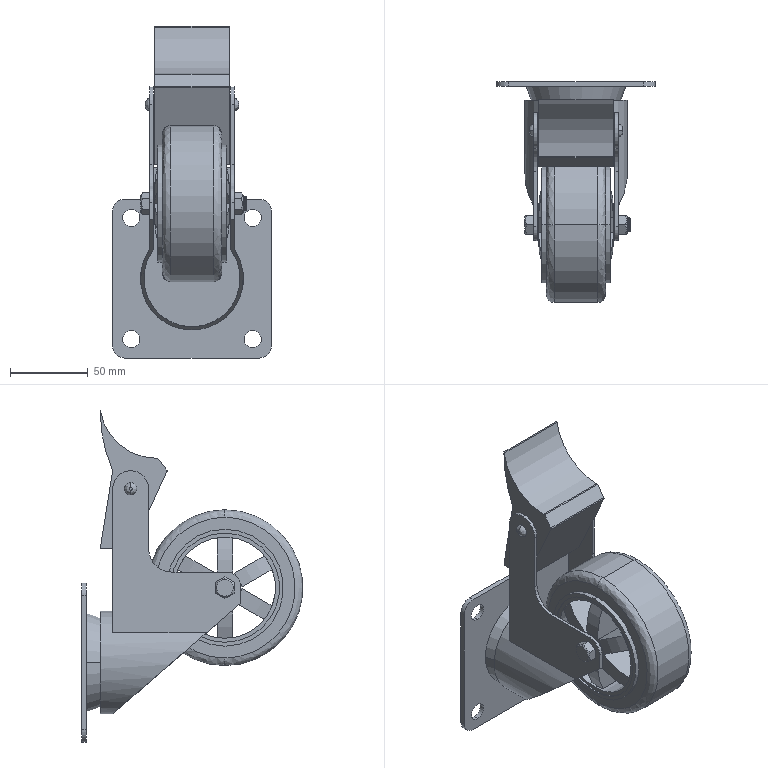Part | SolidWorks | features BaseBody 1 | 1 solid | 150 faces | box 102 x 142 x 213 mm | volume 452222 mm3 | plane 68 | cylinder 64 | spline 10 | cone 8 | commonest cylinder face diameters 106.25 x12 9 x9 11 x8 8 x4 16 x4 70 x4